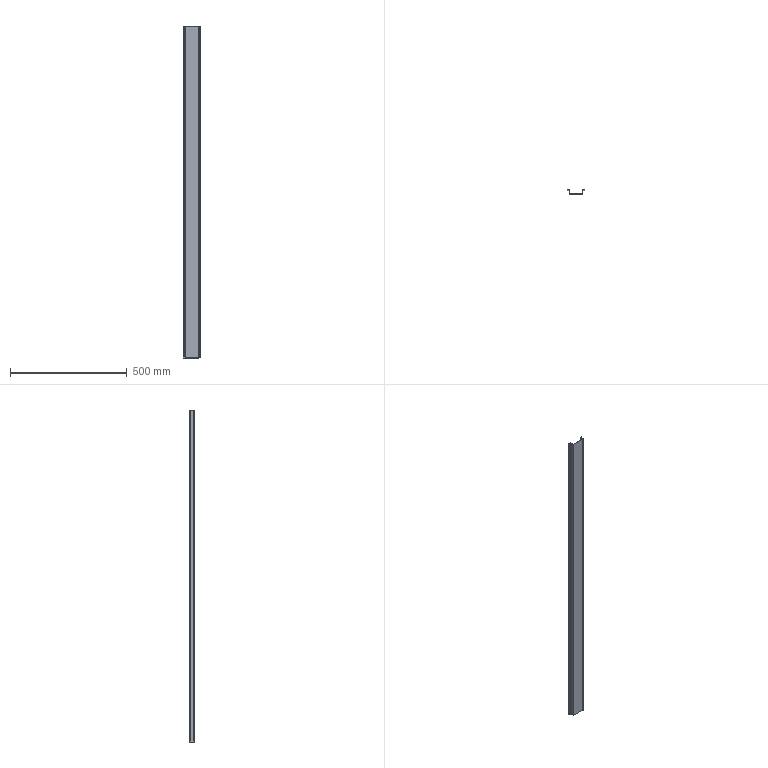Part | SolidWorks | features FlatPattern 1, SMBaseFlange 1, SheetMetal 1 | 1 solid | 38 faces | box 77 x 18 x 1424 mm | volume 231476 mm3 | plane 30 | cylinder 8 | commonest cylinder face diameters 0.4 x4 3.4 x4
STEP:
#1=CARTESIAN_POINT('',(-30.2,16.5,712.));
#2=VERTEX_POINT('',#1);
#3=CARTESIAN_POINT('',(-30.2,18.,712.));
#4=VERTEX_POINT('',#3);
#5=CARTESIAN_POINT('',(-30.2,16.5,712.));
#6=DIRECTION('',(0.,1.,0.));
#7=VECTOR('',#6,1000.);
#8=LINE('',#5,#7);
#9=EDGE_CURVE('',#2,#4,#8,.T.);
#10=ORIENTED_EDGE('',*,*,#9,.F.);
#11=CARTESIAN_POINT('',(-30.,16.3,712.));
#12=VERTEX_POINT('',#11);
#13=CARTESIAN_POINT('',(-30.2,16.3,712.));
#14=DIRECTION('',(0.,0.,-1.));
#15=DIRECTION('',(1.,0.,0.));
#16=AXIS2_PLACEMENT_3D('',#13,#14,#15);
#17=CIRCLE('',#16,0.2);
#18=EDGE_CURVE('',#2,#12,#17,.T.);
#19=ORIENTED_EDGE('',*,*,#18,.T.);
#20=CARTESIAN_POINT('',(-28.5,16.3,712.));
#21=VERTEX_POINT('',#20);
#22=CARTESIAN_POINT('',(-28.5,16.3,712.));
#23=DIRECTION('',(-1.,0.,0.));
#24=VECTOR('',#23,1000.);
#25=LINE('',#22,#24);
#26=EDGE_CURVE('',#21,#12,#25,.T.);
#27=ORIENTED_EDGE('',*,*,#26,.F.);
#28=CARTESIAN_POINT('',(-30.2,16.3,712.));
#29=DIRECTION('',(0.,0.,-1.));
#30=DIRECTION('',(1.,0.,0.));
#31=AXIS2_PLACEMENT_3D('',#28,#29,#30);
#32=CIRCLE('',#31,1.7);
#33=EDGE_CURVE('',#4,#21,#32,.T.);
#34=ORIENTED_EDGE('',*,*,#33,.F.);
#35=EDGE_LOOP('',(#10,#19,#27,#34));
#36=FACE_OUTER_BOUND('',#35,.T.);
#37=CARTESIAN_POINT('',(-30.2,16.5,712.));
#38=DIRECTION('',(0.,0.,1.));
#39=DIRECTION('',(1.,0.,0.));
#40=AXIS2_PLACEMENT_3D('',#37,#38,#39);
#41=PLANE('',#40);
#42=ADVANCED_FACE('',(#36),#41,.T.);
#43=CARTESIAN_POINT('',(-38.5,16.5,712.));
#44=VERTEX_POINT('',#43);
#45=CARTESIAN_POINT('',(-30.,16.5,712.));
#46=DIRECTION('',(1.,0.,0.));
#47=VECTOR('',#46,1000.);
#48=LINE('',#45,#47);
#49=EDGE_CURVE('',#44,#2,#48,.T.);
#50=ORIENTED_EDGE('',*,*,#49,.T.);
#51=ORIENTED_EDGE('',*,*,#9,.T.);
#52=CARTESIAN_POINT('',(-38.5,18.,712.));
#53=VERTEX_POINT('',#52);
#54=CARTESIAN_POINT('',(-30.,18.,712.));
#55=DIRECTION('',(1.,0.,0.));
#56=VECTOR('',#55,1000.);
#57=LINE('',#54,#56);
#58=EDGE_CURVE('',#53,#4,#57,.T.);
#59=ORIENTED_EDGE('',*,*,#58,.F.);
#60=CARTESIAN_POINT('',(-38.5,16.5,712.));
#61=DIRECTION('',(0.,1.,0.));
#62=VECTOR('',#61,1000.);
#63=LINE('',#60,#62);
#64=EDGE_CURVE('',#44,#53,#63,.T.);
#65=ORIENTED_EDGE('',*,*,#64,.F.);
#66=EDGE_LOOP('',(#50,#51,#59,#65));
#67=FACE_OUTER_BOUND('',#66,.T.);
#68=CARTESIAN_POINT('',(-28.5,16.3,712.));
#69=DIRECTION('',(0.,0.,1.));
#70=DIRECTION('',(1.,0.,0.));
#71=AXIS2_PLACEMENT_3D('',#68,#69,#70);
#72=PLANE('',#71);
#73=ADVANCED_FACE('',(#67),#72,.T.);
#74=CARTESIAN_POINT('',(-30.,16.3,-712.));
#75=VERTEX_POINT('',#74);
#76=CARTESIAN_POINT('',(-28.5,16.3,-712.));
#77=VERTEX_POINT('',#76);
#78=CARTESIAN_POINT('',(-30.,16.3,-712.));
#79=DIRECTION('',(1.,0.,0.));
#80=VECTOR('',#79,1000.);
#81=LINE('',#78,#80);
#82=EDGE_CURVE('',#75,#77,#81,.T.);
#83=ORIENTED_EDGE('',*,*,#82,.F.);
#84=CARTESIAN_POINT('',(-30.2,16.5,-712.));
#85=VERTEX_POINT('',#84);
#86=CARTESIAN_POINT('',(-30.2,16.3,-712.));
#87=DIRECTION('',(0.,0.,-1.));
#88=DIRECTION('',(1.,0.,0.));
#89=AXIS2_PLACEMENT_3D('',#86,#87,#88);
#90=CIRCLE('',#89,0.2);
#91=EDGE_CURVE('',#85,#75,#90,.T.);
#92=ORIENTED_EDGE('',*,*,#91,.F.);
#93=CARTESIAN_POINT('',(-30.2,18.,-712.));
#94=VERTEX_POINT('',#93);
#95=CARTESIAN_POINT('',(-30.2,18.,-712.));
#96=DIRECTION('',(0.,-1.,0.));
#97=VECTOR('',#96,1000.);
#98=LINE('',#95,#97);
#99=EDGE_CURVE('',#94,#85,#98,.T.);
#100=ORIENTED_EDGE('',*,*,#99,.F.);
#101=CARTESIAN_POINT('',(-30.2,16.3,-712.));
#102=DIRECTION('',(0.,0.,-1.));
#103=DIRECTION('',(1.,0.,0.));
#104=AXIS2_PLACEMENT_3D('',#101,#102,#103);
#105=CIRCLE('',#104,1.7);
#106=EDGE_CURVE('',#94,#77,#105,.T.);
#107=ORIENTED_EDGE('',*,*,#106,.T.);
#108=EDGE_LOOP('',(#83,#92,#100,#107));
#109=FACE_OUTER_BOUND('',#108,.T.);
#110=CARTESIAN_POINT('',(-30.,16.3,-712.));
#111=DIRECTION('',(0.,0.,-1.));
#112=DIRECTION('',(-1.,0.,0.));
#113=AXIS2_PLACEMENT_3D('',#110,#111,#112);
#114=PLANE('',#113);
#115=ADVANCED_FACE('',(#109),#114,.T.);
#116=CARTESIAN_POINT('',(-30.,1.7,-712.));
#117=VERTEX_POINT('',#116);
#118=CARTESIAN_POINT('',(-30.,16.5,-712.));
#119=DIRECTION('',(0.,-1.,0.));
#120=VECTOR('',#119,1000.);
#121=LINE('',#118,#120);
#122=EDGE_CURVE('',#75,#117,#121,.T.);
#123=ORIENTED_EDGE('',*,*,#122,.F.);
#124=ORIENTED_EDGE('',*,*,#82,.T.);
#125=CARTESIAN_POINT('',(-28.5,1.7,-712.));
#126=VERTEX_POINT('',#125);
#127=CARTESIAN_POINT('',(-28.5,16.5,-712.));
#128=DIRECTION('',(0.,-1.,0.));
#129=VECTOR('',#128,1000.);
#130=LINE('',#127,#129);
#131=EDGE_CURVE('',#77,#126,#130,.T.);
#132=ORIENTED_EDGE('',*,*,#131,.T.);
#133=CARTESIAN_POINT('',(-28.5,1.7,-712.));
#134=DIRECTION('',(-1.,0.,0.));
#135=VECTOR('',#134,1000.);
#136=LINE('',#133,#135);
#137=EDGE_CURVE('',#126,#117,#136,.T.);
#138=ORIENTED_EDGE('',*,*,#137,.T.);
#139=EDGE_LOOP('',(#123,#124,#132,#138));
#140=FACE_OUTER_BOUND('',#139,.T.);
#141=CARTESIAN_POINT('',(-30.2,18.,-712.));
#142=DIRECTION('',(0.,0.,-1.));
#143=DIRECTION('',(-1.,0.,0.));
#144=AXIS2_PLACEMENT_3D('',#141,#142,#143);
#145=PLANE('',#144);
#146=ADVANCED_FACE('',(#140),#145,.T.);
#147=CARTESIAN_POINT('',(-30.,1.7,712.));
#148=VERTEX_POINT('',#147);
#149=CARTESIAN_POINT('',(-28.5,1.7,712.));
#150=VERTEX_POINT('',#149);
#151=CARTESIAN_POINT('',(-30.,1.7,712.));
#152=DIRECTION('',(1.,0.,0.));
#153=VECTOR('',#152,1000.);
#154=LINE('',#151,#153);
#155=EDGE_CURVE('',#148,#150,#154,.T.);
#156=ORIENTED_EDGE('',*,*,#155,.F.);
#157=CARTESIAN_POINT('',(-28.3,0.,712.));
#158=VERTEX_POINT('',#157);
#159=CARTESIAN_POINT('',(-28.3,1.7,712.));
#160=DIRECTION('',(0.,0.,1.));
#161=DIRECTION('',(-1.,0.,0.));
#162=AXIS2_PLACEMENT_3D('',#159,#160,#161);
#163=CIRCLE('',#162,1.7);
#164=EDGE_CURVE('',#148,#158,#163,.T.);
#165=ORIENTED_EDGE('',*,*,#164,.T.);
#166=CARTESIAN_POINT('',(-28.3,1.5,712.));
#167=VERTEX_POINT('',#166);
#168=CARTESIAN_POINT('',(-28.3,1.5,712.));
#169=DIRECTION('',(0.,-1.,0.));
#170=VECTOR('',#169,1000.);
#171=LINE('',#168,#170);
#172=EDGE_CURVE('',#167,#158,#171,.T.);
#173=ORIENTED_EDGE('',*,*,#172,.F.);
#174=CARTESIAN_POINT('',(-28.3,1.7,712.));
#175=DIRECTION('',(0.,0.,1.));
#176=DIRECTION('',(1.,0.,0.));
#177=AXIS2_PLACEMENT_3D('',#174,#175,#176);
#178=CIRCLE('',#177,0.2);
#179=EDGE_CURVE('',#150,#167,#178,.T.);
#180=ORIENTED_EDGE('',*,*,#179,.F.);
#181=EDGE_LOOP('',(#156,#165,#173,#180));
#182=FACE_OUTER_BOUND('',#181,.T.);
#183=CARTESIAN_POINT('',(-30.,1.7,712.));
#184=DIRECTION('',(0.,0.,1.));
#185=DIRECTION('',(1.,0.,0.));
#186=AXIS2_PLACEMENT_3D('',#183,#184,#185);
#187=PLANE('',#186);
#188=ADVANCED_FACE('',(#182),#187,.T.);
#189=CARTESIAN_POINT('',(-30.,16.5,712.));
#190=DIRECTION('',(0.,-1.,0.));
#191=VECTOR('',#190,1000.);
#192=LINE('',#189,#191);
#193=EDGE_CURVE('',#12,#148,#192,.T.);
#194=ORIENTED_EDGE('',*,*,#193,.T.);
#195=ORIENTED_EDGE('',*,*,#155,.T.);
#196=CARTESIAN_POINT('',(-28.5,16.5,712.));
#197=DIRECTION('',(0.,-1.,0.));
#198=VECTOR('',#197,1000.);
#199=LINE('',#196,#198);
#200=EDGE_CURVE('',#21,#150,#199,.T.);
#201=ORIENTED_EDGE('',*,*,#200,.F.);
#202=ORIENTED_EDGE('',*,*,#26,.T.);
#203=EDGE_LOOP('',(#194,#195,#201,#202));
#204=FACE_OUTER_BOUND('',#203,.T.);
#205=CARTESIAN_POINT('',(-28.3,1.5,712.));
#206=DIRECTION('',(0.,0.,1.));
#207=DIRECTION('',(1.,0.,0.));
#208=AXIS2_PLACEMENT_3D('',#205,#206,#207);
#209=PLANE('',#208);
#210=ADVANCED_FACE('',(#204),#209,.T.);
#211=CARTESIAN_POINT('',(-28.3,0.,-712.));
#212=VERTEX_POINT('',#211);
#213=CARTESIAN_POINT('',(-28.3,1.5,-712.));
#214=VERTEX_POINT('',#213);
#215=CARTESIAN_POINT('',(-28.3,0.,-712.));
#216=DIRECTION('',(0.,1.,0.));
#217=VECTOR('',#216,1000.);
#218=LINE('',#215,#217);
#219=EDGE_CURVE('',#212,#214,#218,.T.);
#220=ORIENTED_EDGE('',*,*,#219,.F.);
#221=CARTESIAN_POINT('',(-28.3,1.7,-712.));
#222=DIRECTION('',(0.,0.,1.));
#223=DIRECTION('',(-1.,0.,0.));
#224=AXIS2_PLACEMENT_3D('',#221,#222,#223);
#225=CIRCLE('',#224,1.7);
#226=EDGE_CURVE('',#117,#212,#225,.T.);
#227=ORIENTED_EDGE('',*,*,#226,.F.);
#228=ORIENTED_EDGE('',*,*,#137,.F.);
#229=CARTESIAN_POINT('',(-28.3,1.7,-712.));
#230=DIRECTION('',(0.,0.,1.));
#231=DIRECTION('',(1.,0.,0.));
#232=AXIS2_PLACEMENT_3D('',#229,#230,#231);
#233=CIRCLE('',#232,0.2);
#234=EDGE_CURVE('',#126,#214,#233,.T.);
#235=ORIENTED_EDGE('',*,*,#234,.T.);
#236=EDGE_LOOP('',(#220,#227,#228,#235));
#237=FACE_OUTER_BOUND('',#236,.T.);
#238=CARTESIAN_POINT('',(-28.3,0.,-712.));
#239=DIRECTION('',(0.,0.,-1.));
#240=DIRECTION('',(-1.,0.,0.));
#241=AXIS2_PLACEMENT_3D('',#238,#239,#240);
#242=PLANE('',#241);
#243=ADVANCED_FACE('',(#237),#242,.T.);
#244=CARTESIAN_POINT('',(28.3,0.,-712.));
#245=VERTEX_POINT('',#244);
#246=CARTESIAN_POINT('',(-30.,0.,-712.));
#247=DIRECTION('',(1.,0.,0.));
#248=VECTOR('',#247,1000.);
#249=LINE('',#246,#248);
#250=EDGE_CURVE('',#212,#245,#249,.T.);
#251=ORIENTED_EDGE('',*,*,#250,.F.);
#252=ORIENTED_EDGE('',*,*,#219,.T.);
#253=CARTESIAN_POINT('',(28.3,1.5,-712.));
#254=VERTEX_POINT('',#253);
#255=CARTESIAN_POINT('',(-30.,1.5,-712.));
#256=DIRECTION('',(1.,0.,0.));
#257=VECTOR('',#256,1000.);
#258=LINE('',#255,#257);
#259=EDGE_CURVE('',#214,#254,#258,.T.);
#260=ORIENTED_EDGE('',*,*,#259,.T.);
#261=CARTESIAN_POINT('',(28.3,1.5,-712.));
#262=DIRECTION('',(0.,-1.,0.));
#263=VECTOR('',#262,1000.);
#264=LINE('',#261,#263);
#265=EDGE_CURVE('',#254,#245,#264,.T.);
#266=ORIENTED_EDGE('',*,*,#265,.T.);
#267=EDGE_LOOP('',(#251,#252,#260,#266));
#268=FACE_OUTER_BOUND('',#267,.T.);
#269=CARTESIAN_POINT('',(-28.5,1.7,-712.));
#270=DIRECTION('',(0.,0.,-1.));
#271=DIRECTION('',(-1.,0.,0.));
#272=AXIS2_PLACEMENT_3D('',#269,#270,#271);
#273=PLANE('',#272);
#274=ADVANCED_FACE('',(#268),#273,.T.);
#275=CARTESIAN_POINT('',(28.3,0.,712.));
#276=VERTEX_POINT('',#275);
#277=CARTESIAN_POINT('',(28.3,1.5,712.));
#278=VERTEX_POINT('',#277);
#279=CARTESIAN_POINT('',(28.3,0.,712.));
#280=DIRECTION('',(0.,1.,0.));
#281=VECTOR('',#280,1000.);
#282=LINE('',#279,#281);
#283=EDGE_CURVE('',#276,#278,#282,.T.);
#284=ORIENTED_EDGE('',*,*,#283,.F.);
#285=CARTESIAN_POINT('',(30.,1.7,712.));
#286=VERTEX_POINT('',#285);
#287=CARTESIAN_POINT('',(28.3,1.7,712.));
#288=DIRECTION('',(0.,0.,1.));
#289=DIRECTION('',(-1.,0.,0.));
#290=AXIS2_PLACEMENT_3D('',#287,#288,#289);
#291=CIRCLE('',#290,1.7);
#292=EDGE_CURVE('',#276,#286,#291,.T.);
#293=ORIENTED_EDGE('',*,*,#292,.T.);
#294=CARTESIAN_POINT('',(28.5,1.7,712.));
#295=VERTEX_POINT('',#294);
#296=CARTESIAN_POINT('',(28.5,1.7,712.));
#297=DIRECTION('',(1.,0.,0.));
#298=VECTOR('',#297,1000.);
#299=LINE('',#296,#298);
#300=EDGE_CURVE('',#295,#286,#299,.T.);
#301=ORIENTED_EDGE('',*,*,#300,.F.);
#302=CARTESIAN_POINT('',(28.3,1.7,712.));
#303=DIRECTION('',(0.,0.,1.));
#304=DIRECTION('',(1.,0.,0.));
#305=AXIS2_PLACEMENT_3D('',#302,#303,#304);
#306=CIRCLE('',#305,0.2);
#307=EDGE_CURVE('',#278,#295,#306,.T.);
#308=ORIENTED_EDGE('',*,*,#307,.F.);
#309=EDGE_LOOP('',(#284,#293,#301,#308));
#310=FACE_OUTER_BOUND('',#309,.T.);
#311=CARTESIAN_POINT('',(28.3,0.,712.));
#312=DIRECTION('',(0.,0.,1.));
#313=DIRECTION('',(1.,0.,0.));
#314=AXIS2_PLACEMENT_3D('',#311,#312,#313);
#315=PLANE('',#314);
#316=ADVANCED_FACE('',(#310),#315,.T.);
#317=CARTESIAN_POINT('',(-30.,0.,712.));
#318=DIRECTION('',(1.,0.,0.));
#319=VECTOR('',#318,1000.);
#320=LINE('',#317,#319);
#321=EDGE_CURVE('',#158,#276,#320,.T.);
#322=ORIENTED_EDGE('',*,*,#321,.T.);
#323=ORIENTED_EDGE('',*,*,#283,.T.);
#324=CARTESIAN_POINT('',(-30.,1.5,712.));
#325=DIRECTION('',(1.,0.,0.));
#326=VECTOR('',#325,1000.);
#327=LINE('',#324,#326);
#328=EDGE_CURVE('',#167,#278,#327,.T.);
#329=ORIENTED_EDGE('',*,*,#328,.F.);
#330=ORIENTED_EDGE('',*,*,#172,.T.);
#331=EDGE_LOOP('',(#322,#323,#329,#330));
#332=FACE_OUTER_BOUND('',#331,.T.);
#333=CARTESIAN_POINT('',(28.5,1.7,712.));
#334=DIRECTION('',(0.,0.,1.));
#335=DIRECTION('',(1.,0.,0.));
#336=AXIS2_PLACEMENT_3D('',#333,#334,#335);
#337=PLANE('',#336);
#338=ADVANCED_FACE('',(#332),#337,.T.);
#339=CARTESIAN_POINT('',(30.,1.7,-712.));
#340=VERTEX_POINT('',#339);
#341=CARTESIAN_POINT('',(28.5,1.7,-712.));
#342=VERTEX_POINT('',#341);
#343=CARTESIAN_POINT('',(30.,1.7,-712.));
#344=DIRECTION('',(-1.,0.,0.));
#345=VECTOR('',#344,1000.);
#346=LINE('',#343,#345);
#347=EDGE_CURVE('',#340,#342,#346,.T.);
#348=ORIENTED_EDGE('',*,*,#347,.F.);
#349=CARTESIAN_POINT('',(28.3,1.7,-712.));
#350=DIRECTION('',(0.,0.,1.));
#351=DIRECTION('',(-1.,0.,0.));
#352=AXIS2_PLACEMENT_3D('',#349,#350,#351);
#353=CIRCLE('',#352,1.7);
#354=EDGE_CURVE('',#245,#340,#353,.T.);
#355=ORIENTED_EDGE('',*,*,#354,.F.);
#356=ORIENTED_EDGE('',*,*,#265,.F.);
#357=CARTESIAN_POINT('',(28.3,1.7,-712.));
#358=DIRECTION('',(0.,0.,1.));
#359=DIRECTION('',(1.,0.,0.));
#360=AXIS2_PLACEMENT_3D('',#357,#358,#359);
#361=CIRCLE('',#360,0.2);
#362=EDGE_CURVE('',#254,#342,#361,.T.);
#363=ORIENTED_EDGE('',*,*,#362,.T.);
#364=EDGE_LOOP('',(#348,#355,#356,#363));
#365=FACE_OUTER_BOUND('',#364,.T.);
#366=CARTESIAN_POINT('',(30.,1.7,-712.));
#367=DIRECTION('',(0.,0.,-1.));
#368=DIRECTION('',(-1.,0.,0.));
#369=AXIS2_PLACEMENT_3D('',#366,#367,#368);
#370=PLANE('',#369);
#371=ADVANCED_FACE('',(#365),#370,.T.);
#372=CARTESIAN_POINT('',(30.,16.3,-712.));
#373=VERTEX_POINT('',#372);
#374=CARTESIAN_POINT('',(30.,0.,-712.));
#375=DIRECTION('',(0.,1.,0.));
#376=VECTOR('',#375,1000.);
#377=LINE('',#374,#376);
#378=EDGE_CURVE('',#340,#373,#377,.T.);
#379=ORIENTED_EDGE('',*,*,#378,.F.);
#380=ORIENTED_EDGE('',*,*,#347,.T.);
#381=CARTESIAN_POINT('',(28.5,16.3,-712.));
#382=VERTEX_POINT('',#381);
#383=CARTESIAN_POINT('',(28.5,0.,-712.));
#384=DIRECTION('',(0.,1.,0.));
#385=VECTOR('',#384,1000.);
#386=LINE('',#383,#385);
#387=EDGE_CURVE('',#342,#382,#386,.T.);
#388=ORIENTED_EDGE('',*,*,#387,.T.);
#389=CARTESIAN_POINT('',(28.5,16.3,-712.));
#390=DIRECTION('',(1.,0.,0.));
#391=VECTOR('',#390,1000.);
#392=LINE('',#389,#391);
#393=EDGE_CURVE('',#382,#373,#392,.T.);
#394=ORIENTED_EDGE('',*,*,#393,.T.);
#395=EDGE_LOOP('',(#379,#380,#388,#394));
#396=FACE_OUTER_BOUND('',#395,.T.);
#397=CARTESIAN_POINT('',(28.3,1.5,-712.));
#398=DIRECTION('',(0.,0.,-1.));
#399=DIRECTION('',(-1.,0.,0.));
#400=AXIS2_PLACEMENT_3D('',#397,#398,#399);
#401=PLANE('',#400);
#402=ADVANCED_FACE('',(#396),#401,.T.);
#403=CARTESIAN_POINT('',(30.,16.3,712.));
#404=VERTEX_POINT('',#403);
#405=CARTESIAN_POINT('',(28.5,16.3,712.));
#406=VERTEX_POINT('',#405);
#407=CARTESIAN_POINT('',(30.,16.3,712.));
#408=DIRECTION('',(-1.,0.,0.));
#409=VECTOR('',#408,1000.);
#410=LINE('',#407,#409);
#411=EDGE_CURVE('',#404,#406,#410,.T.);
#412=ORIENTED_EDGE('',*,*,#411,.F.);
#413=CARTESIAN_POINT('',(30.2,16.5,712.));
#414=VERTEX_POINT('',#413);
#415=CARTESIAN_POINT('',(30.2,16.3,712.));
#416=DIRECTION('',(0.,0.,-1.));
#417=DIRECTION('',(1.,0.,0.));
#418=AXIS2_PLACEMENT_3D('',#415,#416,#417);
#419=CIRCLE('',#418,0.2);
#420=EDGE_CURVE('',#404,#414,#419,.T.);
#421=ORIENTED_EDGE('',*,*,#420,.T.);
#422=CARTESIAN_POINT('',(30.2,18.,712.));
#423=VERTEX_POINT('',#422);
#424=CARTESIAN_POINT('',(30.2,18.,712.));
#425=DIRECTION('',(0.,-1.,0.));
#426=VECTOR('',#425,1000.);
#427=LINE('',#424,#426);
#428=EDGE_CURVE('',#423,#414,#427,.T.);
#429=ORIENTED_EDGE('',*,*,#428,.F.);
#430=CARTESIAN_POINT('',(30.2,16.3,712.));
#431=DIRECTION('',(0.,0.,-1.));
#432=DIRECTION('',(1.,0.,0.));
#433=AXIS2_PLACEMENT_3D('',#430,#431,#432);
#434=CIRCLE('',#433,1.7);
#435=EDGE_CURVE('',#406,#423,#434,.T.);
#436=ORIENTED_EDGE('',*,*,#435,.F.);
#437=EDGE_LOOP('',(#412,#421,#429,#436));
#438=FACE_OUTER_BOUND('',#437,.T.);
#439=CARTESIAN_POINT('',(30.,16.3,712.));
#440=DIRECTION('',(0.,0.,1.));
#441=DIRECTION('',(1.,0.,0.));
#442=AXIS2_PLACEMENT_3D('',#439,#440,#441);
#443=PLANE('',#442);
#444=ADVANCED_FACE('',(#438),#443,.T.);
#445=CARTESIAN_POINT('',(30.,0.,712.));
#446=DIRECTION('',(0.,1.,0.));
#447=VECTOR('',#446,1000.);
#448=LINE('',#445,#447);
#449=EDGE_CURVE('',#286,#404,#448,.T.);
#450=ORIENTED_EDGE('',*,*,#449,.T.);
#451=ORIENTED_EDGE('',*,*,#411,.T.);
#452=CARTESIAN_POINT('',(28.5,0.,712.));
#453=DIRECTION('',(0.,1.,0.));
#454=VECTOR('',#453,1000.);
#455=LINE('',#452,#454);
#456=EDGE_CURVE('',#295,#406,#455,.T.);
#457=ORIENTED_EDGE('',*,*,#456,.F.);
#458=ORIENTED_EDGE('',*,*,#300,.T.);
#459=EDGE_LOOP('',(#450,#451,#457,#458));
#460=FACE_OUTER_BOUND('',#459,.T.);
#461=CARTESIAN_POINT('',(30.2,18.,712.));
#462=DIRECTION('',(0.,0.,1.));
#463=DIRECTION('',(1.,0.,0.));
#464=AXIS2_PLACEMENT_3D('',#461,#462,#463);
#465=PLANE('',#464);
#466=ADVANCED_FACE('',(#460),#465,.T.);
#467=CARTESIAN_POINT('',(30.2,16.5,-712.));
#468=VERTEX_POINT('',#467);
#469=CARTESIAN_POINT('',(30.2,18.,-712.));
#470=VERTEX_POINT('',#469);
#471=CARTESIAN_POINT('',(30.2,16.5,-712.));
#472=DIRECTION('',(0.,1.,0.));
#473=VECTOR('',#472,1000.);
#474=LINE('',#471,#473);
#475=EDGE_CURVE('',#468,#470,#474,.T.);
#476=ORIENTED_EDGE('',*,*,#475,.F.);
#477=CARTESIAN_POINT('',(30.2,16.3,-712.));
#478=DIRECTION('',(0.,0.,-1.));
#479=DIRECTION('',(1.,0.,0.));
#480=AXIS2_PLACEMENT_3D('',#477,#478,#479);
#481=CIRCLE('',#480,0.2);
#482=EDGE_CURVE('',#373,#468,#481,.T.);
#483=ORIENTED_EDGE('',*,*,#482,.F.);
#484=ORIENTED_EDGE('',*,*,#393,.F.);
#485=CARTESIAN_POINT('',(30.2,16.3,-712.));
#486=DIRECTION('',(0.,0.,-1.));
#487=DIRECTION('',(1.,0.,0.));
#488=AXIS2_PLACEMENT_3D('',#485,#486,#487);
#489=CIRCLE('',#488,1.7);
#490=EDGE_CURVE('',#382,#470,#489,.T.);
#491=ORIENTED_EDGE('',*,*,#490,.T.);
#492=EDGE_LOOP('',(#476,#483,#484,#491));
#493=FACE_OUTER_BOUND('',#492,.T.);
#494=CARTESIAN_POINT('',(30.2,16.5,-712.));
#495=DIRECTION('',(0.,0.,-1.));
#496=DIRECTION('',(-1.,0.,0.));
#497=AXIS2_PLACEMENT_3D('',#494,#495,#496);
#498=PLANE('',#497);
#499=ADVANCED_FACE('',(#493),#498,.T.);
#500=CARTESIAN_POINT('',(38.5,16.5,-712.));
#501=VERTEX_POINT('',#500);
#502=CARTESIAN_POINT('',(30.,16.5,-712.));
#503=DIRECTION('',(1.,0.,0.));
#504=VECTOR('',#503,1000.);
#505=LINE('',#502,#504);
#506=EDGE_CURVE('',#468,#501,#505,.T.);
#507=ORIENTED_EDGE('',*,*,#506,.F.);
#508=ORIENTED_EDGE('',*,*,#475,.T.);
#509=CARTESIAN_POINT('',(38.5,18.,-712.));
#510=VERTEX_POINT('',#509);
#511=CARTESIAN_POINT('',(30.,18.,-712.));
#512=DIRECTION('',(1.,0.,0.));
#513=VECTOR('',#512,1000.);
#514=LINE('',#511,#513);
#515=EDGE_CURVE('',#470,#510,#514,.T.);
#516=ORIENTED_EDGE('',*,*,#515,.T.);
#517=CARTESIAN_POINT('',(38.5,18.,-712.));
#518=DIRECTION('',(0.,-1.,0.));
#519=VECTOR('',#518,1000.);
#520=LINE('',#517,#519);
#521=EDGE_CURVE('',#510,#501,#520,.T.);
#522=ORIENTED_EDGE('',*,*,#521,.T.);
#523=EDGE_LOOP('',(#507,#508,#516,#522));
#524=FACE_OUTER_BOUND('',#523,.T.);
#525=CARTESIAN_POINT('',(28.5,16.3,-712.));
#526=DIRECTION('',(0.,0.,-1.));
#527=DIRECTION('',(-1.,0.,0.));
#528=AXIS2_PLACEMENT_3D('',#525,#526,#527);
#529=PLANE('',#528);
#530=ADVANCED_FACE('',(#524),#529,.T.);
#531=ORIENTED_EDGE('',*,*,#506,.T.);
#532=CARTESIAN_POINT('',(38.5,16.5,712.));
#533=VERTEX_POINT('',#532);
#534=CARTESIAN_POINT('',(38.5,16.5,712.));
#535=DIRECTION('',(0.,0.,-1.));
#536=VECTOR('',#535,1000.);
#537=LINE('',#534,#536);
#538=EDGE_CURVE('',#533,#501,#537,.T.);
#539=ORIENTED_EDGE('',*,*,#538,.F.);
#540=CARTESIAN_POINT('',(30.,16.5,712.));
#541=DIRECTION('',(1.,0.,0.));
#542=VECTOR('',#541,1000.);
#543=LINE('',#540,#542);
#544=EDGE_CURVE('',#414,#533,#543,.T.);
#545=ORIENTED_EDGE('',*,*,#544,.F.);
#546=CARTESIAN_POINT('',(30.2,16.5,712.));
#547=DIRECTION('',(0.,0.,-1.));
#548=VECTOR('',#547,1000.);
#549=LINE('',#546,#548);
#550=EDGE_CURVE('',#414,#468,#549,.T.);
#551=ORIENTED_EDGE('',*,*,#550,.T.);
#552=EDGE_LOOP('',(#531,#539,#545,#551));
#553=FACE_OUTER_BOUND('',#552,.T.);
#554=CARTESIAN_POINT('',(30.,16.5,712.));
#555=DIRECTION('',(0.,1.,0.));
#556=DIRECTION('',(-1.,0.,0.));
#557=AXIS2_PLACEMENT_3D('',#554,#555,#556);
#558=PLANE('',#557);
#559=ADVANCED_FACE('',(#553),#558,.F.);
#560=ORIENTED_EDGE('',*,*,#521,.F.);
#561=CARTESIAN_POINT('',(38.5,18.,712.));
#562=VERTEX_POINT('',#561);
#563=CARTESIAN_POINT('',(38.5,18.,712.));
#564=DIRECTION('',(0.,0.,-1.));
#565=VECTOR('',#564,1000.);
#566=LINE('',#563,#565);
#567=EDGE_CURVE('',#562,#510,#566,.T.);
#568=ORIENTED_EDGE('',*,*,#567,.F.);
#569=CARTESIAN_POINT('',(38.5,18.,712.));
#570=DIRECTION('',(0.,-1.,0.));
#571=VECTOR('',#570,1000.);
#572=LINE('',#569,#571);
#573=EDGE_CURVE('',#562,#533,#572,.T.);
#574=ORIENTED_EDGE('',*,*,#573,.T.);
#575=ORIENTED_EDGE('',*,*,#538,.T.);
#576=EDGE_LOOP('',(#560,#568,#574,#575));
#577=FACE_OUTER_BOUND('',#576,.T.);
#578=CARTESIAN_POINT('',(38.5,18.,712.));
#579=DIRECTION('',(1.,0.,0.));
#580=DIRECTION('',(0.,0.,-1.));
#581=AXIS2_PLACEMENT_3D('',#578,#579,#580);
#582=PLANE('',#581);
#583=ADVANCED_FACE('',(#577),#582,.T.);
#584=ORIENTED_EDGE('',*,*,#515,.F.);
#585=CARTESIAN_POINT('',(30.2,18.,712.));
#586=DIRECTION('',(0.,0.,-1.));
#587=VECTOR('',#586,1000.);
#588=LINE('',#585,#587);
#589=EDGE_CURVE('',#423,#470,#588,.T.);
#590=ORIENTED_EDGE('',*,*,#589,.F.);
#591=CARTESIAN_POINT('',(30.,18.,712.));
#592=DIRECTION('',(1.,0.,0.));
#593=VECTOR('',#592,1000.);
#594=LINE('',#591,#593);
#595=EDGE_CURVE('',#423,#562,#594,.T.);
#596=ORIENTED_EDGE('',*,*,#595,.T.);
#597=ORIENTED_EDGE('',*,*,#567,.T.);
#598=EDGE_LOOP('',(#584,#590,#596,#597));
#599=FACE_OUTER_BOUND('',#598,.T.);
#600=CARTESIAN_POINT('',(30.,18.,712.));
#601=DIRECTION('',(0.,1.,0.));
#602=DIRECTION('',(-1.,0.,0.));
#603=AXIS2_PLACEMENT_3D('',#600,#601,#602);
#604=PLANE('',#603);
#605=ADVANCED_FACE('',(#599),#604,.T.);
#606=ORIENTED_EDGE('',*,*,#490,.F.);
#607=CARTESIAN_POINT('',(28.5,16.3,712.));
#608=DIRECTION('',(0.,0.,-1.));
#609=VECTOR('',#608,1000.);
#610=LINE('',#607,#609);
#611=EDGE_CURVE('',#406,#382,#610,.T.);
#612=ORIENTED_EDGE('',*,*,#611,.F.);
#613=ORIENTED_EDGE('',*,*,#435,.T.);
#614=ORIENTED_EDGE('',*,*,#589,.T.);
#615=EDGE_LOOP('',(#606,#612,#613,#614));
#616=FACE_OUTER_BOUND('',#615,.T.);
#617=CARTESIAN_POINT('',(30.2,16.3,712.));
#618=DIRECTION('',(0.,0.,-1.));
#619=DIRECTION('',(-1.,0.,0.));
#620=AXIS2_PLACEMENT_3D('',#617,#618,#619);
#621=CYLINDRICAL_SURFACE('',#620,1.7);
#622=ADVANCED_FACE('',(#616),#621,.T.);
#623=ORIENTED_EDGE('',*,*,#387,.F.);
#624=CARTESIAN_POINT('',(28.5,1.7,712.));
#625=DIRECTION('',(0.,0.,-1.));
#626=VECTOR('',#625,1000.);
#627=LINE('',#624,#626);
#628=EDGE_CURVE('',#295,#342,#627,.T.);
#629=ORIENTED_EDGE('',*,*,#628,.F.);
#630=ORIENTED_EDGE('',*,*,#456,.T.);
#631=ORIENTED_EDGE('',*,*,#611,.T.);
#632=EDGE_LOOP('',(#623,#629,#630,#631));
#633=FACE_OUTER_BOUND('',#632,.T.);
#634=CARTESIAN_POINT('',(28.5,0.,712.));
#635=DIRECTION('',(-1.,0.,0.));
#636=DIRECTION('',(0.,0.,1.));
#637=AXIS2_PLACEMENT_3D('',#634,#635,#636);
#638=PLANE('',#637);
#639=ADVANCED_FACE('',(#633),#638,.T.);
#640=ORIENTED_EDGE('',*,*,#362,.F.);
#641=CARTESIAN_POINT('',(28.3,1.5,712.));
#642=DIRECTION('',(0.,0.,-1.));
#643=VECTOR('',#642,1000.);
#644=LINE('',#641,#643);
#645=EDGE_CURVE('',#278,#254,#644,.T.);
#646=ORIENTED_EDGE('',*,*,#645,.F.);
#647=ORIENTED_EDGE('',*,*,#307,.T.);
#648=ORIENTED_EDGE('',*,*,#628,.T.);
#649=EDGE_LOOP('',(#640,#646,#647,#648));
#650=FACE_OUTER_BOUND('',#649,.T.);
#651=CARTESIAN_POINT('',(28.3,1.7,712.));
#652=DIRECTION('',(0.,0.,-1.));
#653=DIRECTION('',(-1.,0.,0.));
#654=AXIS2_PLACEMENT_3D('',#651,#652,#653);
#655=CYLINDRICAL_SURFACE('',#654,0.2);
#656=ADVANCED_FACE('',(#650),#655,.F.);
#657=ORIENTED_EDGE('',*,*,#259,.F.);
#658=CARTESIAN_POINT('',(-28.3,1.5,712.));
#659=DIRECTION('',(0.,0.,-1.));
#660=VECTOR('',#659,1000.);
#661=LINE('',#658,#660);
#662=EDGE_CURVE('',#167,#214,#661,.T.);
#663=ORIENTED_EDGE('',*,*,#662,.F.);
#664=ORIENTED_EDGE('',*,*,#328,.T.);
#665=ORIENTED_EDGE('',*,*,#645,.T.);
#666=EDGE_LOOP('',(#657,#663,#664,#665));
#667=FACE_OUTER_BOUND('',#666,.T.);
#668=CARTESIAN_POINT('',(-30.,1.5,712.));
#669=DIRECTION('',(0.,1.,0.));
#670=DIRECTION('',(0.,0.,1.));
#671=AXIS2_PLACEMENT_3D('',#668,#669,#670);
#672=PLANE('',#671);
#673=ADVANCED_FACE('',(#667),#672,.T.);
#674=ORIENTED_EDGE('',*,*,#234,.F.);
#675=CARTESIAN_POINT('',(-28.5,1.7,712.));
#676=DIRECTION('',(0.,0.,-1.));
#677=VECTOR('',#676,1000.);
#678=LINE('',#675,#677);
#679=EDGE_CURVE('',#150,#126,#678,.T.);
#680=ORIENTED_EDGE('',*,*,#679,.F.);
#681=ORIENTED_EDGE('',*,*,#179,.T.);
#682=ORIENTED_EDGE('',*,*,#662,.T.);
#683=EDGE_LOOP('',(#674,#680,#681,#682));
#684=FACE_OUTER_BOUND('',#683,.T.);
#685=CARTESIAN_POINT('',(-28.3,1.7,712.));
#686=DIRECTION('',(0.,0.,-1.));
#687=DIRECTION('',(-1.,0.,0.));
#688=AXIS2_PLACEMENT_3D('',#685,#686,#687);
#689=CYLINDRICAL_SURFACE('',#688,0.2);
#690=ADVANCED_FACE('',(#684),#689,.F.);
#691=ORIENTED_EDGE('',*,*,#131,.F.);
#692=CARTESIAN_POINT('',(-28.5,16.3,712.));
#693=DIRECTION('',(0.,0.,-1.));
#694=VECTOR('',#693,1000.);
#695=LINE('',#692,#694);
#696=EDGE_CURVE('',#21,#77,#695,.T.);
#697=ORIENTED_EDGE('',*,*,#696,.F.);
#698=ORIENTED_EDGE('',*,*,#200,.T.);
#699=ORIENTED_EDGE('',*,*,#679,.T.);
#700=EDGE_LOOP('',(#691,#697,#698,#699));
#701=FACE_OUTER_BOUND('',#700,.T.);
#702=CARTESIAN_POINT('',(-28.5,16.5,712.));
#703=DIRECTION('',(1.,0.,0.));
#704=DIRECTION('',(0.,0.,-1.));
#705=AXIS2_PLACEMENT_3D('',#702,#703,#704);
#706=PLANE('',#705);
#707=ADVANCED_FACE('',(#701),#706,.T.);
#708=ORIENTED_EDGE('',*,*,#106,.F.);
#709=CARTESIAN_POINT('',(-30.2,18.,712.));
#710=DIRECTION('',(0.,0.,-1.));
#711=VECTOR('',#710,1000.);
#712=LINE('',#709,#711);
#713=EDGE_CURVE('',#4,#94,#712,.T.);
#714=ORIENTED_EDGE('',*,*,#713,.F.);
#715=ORIENTED_EDGE('',*,*,#33,.T.);
#716=ORIENTED_EDGE('',*,*,#696,.T.);
#717=EDGE_LOOP('',(#708,#714,#715,#716));
#718=FACE_OUTER_BOUND('',#717,.T.);
#719=CARTESIAN_POINT('',(-30.2,16.3,712.));
#720=DIRECTION('',(0.,0.,-1.));
#721=DIRECTION('',(-1.,0.,0.));
#722=AXIS2_PLACEMENT_3D('',#719,#720,#721);
#723=CYLINDRICAL_SURFACE('',#722,1.7);
#724=ADVANCED_FACE('',(#718),#723,.T.);
#725=CARTESIAN_POINT('',(-38.5,18.,-712.));
#726=VERTEX_POINT('',#725);
#727=CARTESIAN_POINT('',(-30.,18.,-712.));
#728=DIRECTION('',(1.,0.,0.));
#729=VECTOR('',#728,1000.);
#730=LINE('',#727,#729);
#731=EDGE_CURVE('',#726,#94,#730,.T.);
#732=ORIENTED_EDGE('',*,*,#731,.F.);
#733=CARTESIAN_POINT('',(-38.5,18.,712.));
#734=DIRECTION('',(0.,0.,-1.));
#735=VECTOR('',#734,1000.);
#736=LINE('',#733,#735);
#737=EDGE_CURVE('',#53,#726,#736,.T.);
#738=ORIENTED_EDGE('',*,*,#737,.F.);
#739=ORIENTED_EDGE('',*,*,#58,.T.);
#740=ORIENTED_EDGE('',*,*,#713,.T.);
#741=EDGE_LOOP('',(#732,#738,#739,#740));
#742=FACE_OUTER_BOUND('',#741,.T.);
#743=CARTESIAN_POINT('',(-30.,18.,712.));
#744=DIRECTION('',(0.,1.,0.));
#745=DIRECTION('',(-1.,0.,0.));
#746=AXIS2_PLACEMENT_3D('',#743,#744,#745);
#747=PLANE('',#746);
#748=ADVANCED_FACE('',(#742),#747,.T.);
#749=CARTESIAN_POINT('',(-38.5,16.5,-712.));
#750=VERTEX_POINT('',#749);
#751=CARTESIAN_POINT('',(-38.5,16.5,-712.));
#752=DIRECTION('',(0.,1.,0.));
#753=VECTOR('',#752,1000.);
#754=LINE('',#751,#753);
#755=EDGE_CURVE('',#750,#726,#754,.T.);
#756=ORIENTED_EDGE('',*,*,#755,.F.);
#757=CARTESIAN_POINT('',(-38.5,16.5,712.));
#758=DIRECTION('',(0.,0.,-1.));
#759=VECTOR('',#758,1000.);
#760=LINE('',#757,#759);
#761=EDGE_CURVE('',#44,#750,#760,.T.);
#762=ORIENTED_EDGE('',*,*,#761,.F.);
#763=ORIENTED_EDGE('',*,*,#64,.T.);
#764=ORIENTED_EDGE('',*,*,#737,.T.);
#765=EDGE_LOOP('',(#756,#762,#763,#764));
#766=FACE_OUTER_BOUND('',#765,.T.);
#767=CARTESIAN_POINT('',(-38.5,16.5,712.));
#768=DIRECTION('',(-1.,0.,0.));
#769=DIRECTION('',(0.,0.,1.));
#770=AXIS2_PLACEMENT_3D('',#767,#768,#769);
#771=PLANE('',#770);
#772=ADVANCED_FACE('',(#766),#771,.T.);
#773=CARTESIAN_POINT('',(-30.,16.5,-712.));
#774=DIRECTION('',(1.,0.,0.));
#775=VECTOR('',#774,1000.);
#776=LINE('',#773,#775);
#777=EDGE_CURVE('',#750,#85,#776,.T.);
#778=ORIENTED_EDGE('',*,*,#777,.T.);
#779=CARTESIAN_POINT('',(-30.2,16.5,712.));
#780=DIRECTION('',(0.,0.,-1.));
#781=VECTOR('',#780,1000.);
#782=LINE('',#779,#781);
#783=EDGE_CURVE('',#2,#85,#782,.T.);
#784=ORIENTED_EDGE('',*,*,#783,.F.);
#785=ORIENTED_EDGE('',*,*,#49,.F.);
#786=ORIENTED_EDGE('',*,*,#761,.T.);
#787=EDGE_LOOP('',(#778,#784,#785,#786));
#788=FACE_OUTER_BOUND('',#787,.T.);
#789=CARTESIAN_POINT('',(-30.,16.5,712.));
#790=DIRECTION('',(0.,1.,0.));
#791=DIRECTION('',(-1.,0.,0.));
#792=AXIS2_PLACEMENT_3D('',#789,#790,#791);
#793=PLANE('',#792);
#794=ADVANCED_FACE('',(#788),#793,.F.);
#795=ORIENTED_EDGE('',*,*,#91,.T.);
#796=CARTESIAN_POINT('',(-30.,16.3,712.));
#797=DIRECTION('',(0.,0.,-1.));
#798=VECTOR('',#797,1000.);
#799=LINE('',#796,#798);
#800=EDGE_CURVE('',#12,#75,#799,.T.);
#801=ORIENTED_EDGE('',*,*,#800,.F.);
#802=ORIENTED_EDGE('',*,*,#18,.F.);
#803=ORIENTED_EDGE('',*,*,#783,.T.);
#804=EDGE_LOOP('',(#795,#801,#802,#803));
#805=FACE_OUTER_BOUND('',#804,.T.);
#806=CARTESIAN_POINT('',(-30.2,16.3,712.));
#807=DIRECTION('',(0.,0.,-1.));
#808=DIRECTION('',(-1.,0.,0.));
#809=AXIS2_PLACEMENT_3D('',#806,#807,#808);
#810=CYLINDRICAL_SURFACE('',#809,0.2);
#811=ADVANCED_FACE('',(#805),#810,.F.);
#812=ORIENTED_EDGE('',*,*,#122,.T.);
#813=CARTESIAN_POINT('',(-30.,1.7,712.));
#814=DIRECTION('',(0.,0.,-1.));
#815=VECTOR('',#814,1000.);
#816=LINE('',#813,#815);
#817=EDGE_CURVE('',#148,#117,#816,.T.);
#818=ORIENTED_EDGE('',*,*,#817,.F.);
#819=ORIENTED_EDGE('',*,*,#193,.F.);
#820=ORIENTED_EDGE('',*,*,#800,.T.);
#821=EDGE_LOOP('',(#812,#818,#819,#820));
#822=FACE_OUTER_BOUND('',#821,.T.);
#823=CARTESIAN_POINT('',(-30.,16.5,712.));
#824=DIRECTION('',(1.,0.,0.));
#825=DIRECTION('',(0.,0.,-1.));
#826=AXIS2_PLACEMENT_3D('',#823,#824,#825);
#827=PLANE('',#826);
#828=ADVANCED_FACE('',(#822),#827,.F.);
#829=ORIENTED_EDGE('',*,*,#226,.T.);
#830=CARTESIAN_POINT('',(-28.3,0.,712.));
#831=DIRECTION('',(0.,0.,-1.));
#832=VECTOR('',#831,1000.);
#833=LINE('',#830,#832);
#834=EDGE_CURVE('',#158,#212,#833,.T.);
#835=ORIENTED_EDGE('',*,*,#834,.F.);
#836=ORIENTED_EDGE('',*,*,#164,.F.);
#837=ORIENTED_EDGE('',*,*,#817,.T.);
#838=EDGE_LOOP('',(#829,#835,#836,#837));
#839=FACE_OUTER_BOUND('',#838,.T.);
#840=CARTESIAN_POINT('',(-28.3,1.7,712.));
#841=DIRECTION('',(0.,0.,-1.));
#842=DIRECTION('',(-1.,0.,0.));
#843=AXIS2_PLACEMENT_3D('',#840,#841,#842);
#844=CYLINDRICAL_SURFACE('',#843,1.7);
#845=ADVANCED_FACE('',(#839),#844,.T.);
#846=ORIENTED_EDGE('',*,*,#250,.T.);
#847=CARTESIAN_POINT('',(28.3,0.,712.));
#848=DIRECTION('',(0.,0.,-1.));
#849=VECTOR('',#848,1000.);
#850=LINE('',#847,#849);
#851=EDGE_CURVE('',#276,#245,#850,.T.);
#852=ORIENTED_EDGE('',*,*,#851,.F.);
#853=ORIENTED_EDGE('',*,*,#321,.F.);
#854=ORIENTED_EDGE('',*,*,#834,.T.);
#855=EDGE_LOOP('',(#846,#852,#853,#854));
#856=FACE_OUTER_BOUND('',#855,.T.);
#857=CARTESIAN_POINT('',(-30.,0.,712.));
#858=DIRECTION('',(0.,1.,0.));
#859=DIRECTION('',(0.,0.,1.));
#860=AXIS2_PLACEMENT_3D('',#857,#858,#859);
#861=PLANE('',#860);
#862=ADVANCED_FACE('',(#856),#861,.F.);
#863=ORIENTED_EDGE('',*,*,#354,.T.);
#864=CARTESIAN_POINT('',(30.,1.7,712.));
#865=DIRECTION('',(0.,0.,-1.));
#866=VECTOR('',#865,1000.);
#867=LINE('',#864,#866);
#868=EDGE_CURVE('',#286,#340,#867,.T.);
#869=ORIENTED_EDGE('',*,*,#868,.F.);
#870=ORIENTED_EDGE('',*,*,#292,.F.);
#871=ORIENTED_EDGE('',*,*,#851,.T.);
#872=EDGE_LOOP('',(#863,#869,#870,#871));
#873=FACE_OUTER_BOUND('',#872,.T.);
#874=CARTESIAN_POINT('',(28.3,1.7,712.));
#875=DIRECTION('',(0.,0.,-1.));
#876=DIRECTION('',(-1.,0.,0.));
#877=AXIS2_PLACEMENT_3D('',#874,#875,#876);
#878=CYLINDRICAL_SURFACE('',#877,1.7);
#879=ADVANCED_FACE('',(#873),#878,.T.);
#880=ORIENTED_EDGE('',*,*,#378,.T.);
#881=CARTESIAN_POINT('',(30.,16.3,712.));
#882=DIRECTION('',(0.,0.,-1.));
#883=VECTOR('',#882,1000.);
#884=LINE('',#881,#883);
#885=EDGE_CURVE('',#404,#373,#884,.T.);
#886=ORIENTED_EDGE('',*,*,#885,.F.);
#887=ORIENTED_EDGE('',*,*,#449,.F.);
#888=ORIENTED_EDGE('',*,*,#868,.T.);
#889=EDGE_LOOP('',(#880,#886,#887,#888));
#890=FACE_OUTER_BOUND('',#889,.T.);
#891=CARTESIAN_POINT('',(30.,0.,712.));
#892=DIRECTION('',(-1.,0.,0.));
#893=DIRECTION('',(0.,0.,1.));
#894=AXIS2_PLACEMENT_3D('',#891,#892,#893);
#895=PLANE('',#894);
#896=ADVANCED_FACE('',(#890),#895,.F.);
#897=ORIENTED_EDGE('',*,*,#482,.T.);
#898=ORIENTED_EDGE('',*,*,#550,.F.);
#899=ORIENTED_EDGE('',*,*,#420,.F.);
#900=ORIENTED_EDGE('',*,*,#885,.T.);
#901=EDGE_LOOP('',(#897,#898,#899,#900));
#902=FACE_OUTER_BOUND('',#901,.T.);
#903=CARTESIAN_POINT('',(30.2,16.3,712.));
#904=DIRECTION('',(0.,0.,-1.));
#905=DIRECTION('',(-1.,0.,0.));
#906=AXIS2_PLACEMENT_3D('',#903,#904,#905);
#907=CYLINDRICAL_SURFACE('',#906,0.2);
#908=ADVANCED_FACE('',(#902),#907,.F.);
#909=ORIENTED_EDGE('',*,*,#544,.T.);
#910=ORIENTED_EDGE('',*,*,#573,.F.);
#911=ORIENTED_EDGE('',*,*,#595,.F.);
#912=ORIENTED_EDGE('',*,*,#428,.T.);
#913=EDGE_LOOP('',(#909,#910,#911,#912));
#914=FACE_OUTER_BOUND('',#913,.T.);
#915=CARTESIAN_POINT('',(30.2,16.3,712.));
#916=DIRECTION('',(0.,0.,1.));
#917=DIRECTION('',(1.,0.,0.));
#918=AXIS2_PLACEMENT_3D('',#915,#916,#917);
#919=PLANE('',#918);
#920=ADVANCED_FACE('',(#914),#919,.T.);
#921=ORIENTED_EDGE('',*,*,#731,.T.);
#922=ORIENTED_EDGE('',*,*,#99,.T.);
#923=ORIENTED_EDGE('',*,*,#777,.F.);
#924=ORIENTED_EDGE('',*,*,#755,.T.);
#925=EDGE_LOOP('',(#921,#922,#923,#924));
#926=FACE_OUTER_BOUND('',#925,.T.);
#927=CARTESIAN_POINT('',(30.2,16.3,-712.));
#928=DIRECTION('',(0.,0.,1.));
#929=DIRECTION('',(1.,0.,0.));
#930=AXIS2_PLACEMENT_3D('',#927,#928,#929);
#931=PLANE('',#930);
#932=ADVANCED_FACE('',(#926),#931,.F.);
#933=CLOSED_SHELL('',(#42,#73,#115,#146,#188,#210,#243,#274,#316,#338,#371,#402,#444,#466,#499,#530,#559,#583,#605,#622,#639,#656,#673,#690,#707,#724,#748,#772,#794,#811,#828,#845,#862,#879,#896,#908,#920,#932));
#934=MANIFOLD_SOLID_BREP('',#933);
#935=CARTESIAN_POINT('',(0.,0.,0.));
#936=DIRECTION('',(0.,0.,1.));
#937=DIRECTION('',(1.,0.,0.));
#938=AXIS2_PLACEMENT_3D('',#935,#936,#937);
#939=(LENGTH_UNIT()NAMED_UNIT(*)SI_UNIT(.MILLI.,.METRE.));
#940=UNCERTAINTY_MEASURE_WITH_UNIT(LENGTH_MEASURE(0.00001),#939,'','');
#941=(NAMED_UNIT(*)PLANE_ANGLE_UNIT()SI_UNIT($,.RADIAN.));
#942=(NAMED_UNIT(*)SI_UNIT($,.STERADIAN.)SOLID_ANGLE_UNIT());
#943=(GEOMETRIC_REPRESENTATION_CONTEXT(3)GLOBAL_UNCERTAINTY_ASSIGNED_CONTEXT((#940))GLOBAL_UNIT_ASSIGNED_CONTEXT((#939,#941,#942))REPRESENTATION_CONTEXT('',''));
#944=ADVANCED_BREP_SHAPE_REPRESENTATION('',(#934,#938),#943);